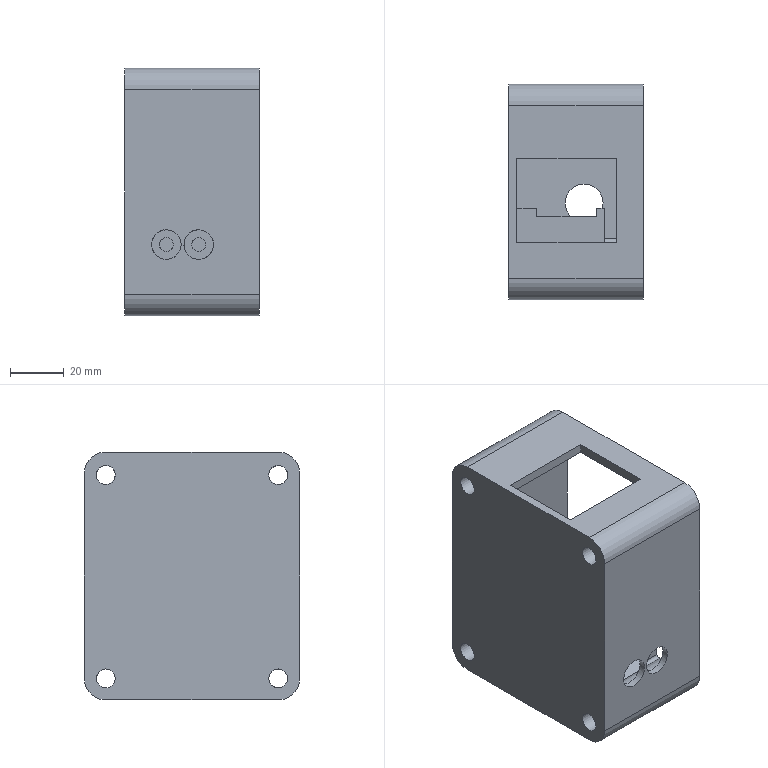NC program | NX | posted by the shop | part box 50 x 80 x 92 mm
Lines 6023 to 6904 of 30419:
(T=7 N=D6-18-D6-50-3T-rough D=6.00 R=0.00 FL=18.00 L=50.00)
(XY-STOCK=0.20)
T7 M6
T11
G0 G90 G54 X34.33 Y-2.568 S4500 M3
G43 H07 Z30.
M8
Z-12.6
G1 X34.203 Y-2.647 Z-13.537 F1500.
X34.075 Y-2.726 Z-13.908
X33.948 Y-2.805 Z-14.18
X33.821 Y-2.884 Z-14.4
X33.693 Y-2.964 Z-14.584
X33.566 Y-3.043 Z-14.742
X33.438 Y-3.122 Z-14.88
X33.311 Y-3.201 Z-15.
X33.184 Y-3.28 Z-15.105
X33.056 Y-3.359 Z-15.198
X32.929 Y-3.439 Z-15.279
X32.801 Y-3.518 Z-15.35
X32.674 Y-3.597 Z-15.41
X32.547 Y-3.676 Z-15.462
X32.419 Y-3.755 Z-15.505
X32.292 Y-3.834 Z-15.539
X32.164 Y-3.914 Z-15.566
X32.037 Y-3.993 Z-15.585
X31.91 Y-4.072 Z-15.596
X31.782 Y-4.151 Z-15.6
X31.004 Y-4.635
G3 X30.803 Y-5.459 I.32 J-.515
X32.656 Y-6.958 I2.88 J1.665
X38.298 Y-4.177 I1.507 J4.056
G1 X38.3 Y-4.147
G3 X38.03 Y-3.647 I-.602 J-.001
G1 X37.795 Y-3.491
X36.799 Y-2.834 Z-15.5
G2 X36.474 Y-2.534 I.395 J.753 F10000.
G1 X36.422 Y-2.396
X36.402 Y-2.25
Y-2.047
X36.411 Y-1.845
G2 X36.787 Y-1.388 I.593 J-.104
X37.582 Y-1.786 Z-15.584 I.214 J-.566 F1500.
G1 X37.649 Y-1.968 Z-15.6
X38.284 Y-3.706
G2 X37.886 Y-5.225 I-2.13 J-.254
X31.206 Y-6.114 I-3.701 J2.265
X30.611 Y-5.298 I1.747 J1.898
X31.515 Y-4.65 I.583 J.141
X31.777 Y-4.97 Z-15.565 I-.44 J-.627
G1 X32.153 Y-5.646 Z-15.5
G3 X33.295 Y-5.298 I.55 J.243 F10000.
X32.764 Y-4.733 I-.618 J-.049
G1 X32.009 Y-4.64
X31.594 Y-4.587 Z-15.535 F1500.
X31.177 Y-4.544 Z-15.57
G3 X30.845 Y-4.655 Z-15.6 I.025 J-.629
X30.598 Y-5.222 I.349 J-.49
X31.213 Y-6.254 I1.851 J.405
X37.298 Y-6.14 I2.983 J3.241
X38.299 Y-4.544 I-2.18 J2.479
G1 X38.3 Y-4.168
G2 X37.808 Y-5.653 I-2.067 J-.138
X31.244 Y-6.371 I-3.609 J2.636
X30.634 Y-5.49 I1.506 J1.696
X31.506 Y-4.849 I.59 J.112
X31.8 Y-5.176 Z-15.563 I-.368 J-.626
G1 X32.174 Y-5.821 Z-15.5
G3 X33.318 Y-5.49 I.546 J.254 F10000.
G1 X33.292 Y-5.303
X33.234 Y-5.122
G3 X32.763 Y-4.797 I-.537 J-.273
G1 X32.036 Y-4.719
X31.184 Y-4.634 Z-15.572 F1500.
G3 X30.868 Y-4.737 Z-15.6 I.031 J-.633
X30.609 Y-5.312 I.338 J-.498
X31.31 Y-6.555 I1.834 J.215
X36.925 Y-6.697 I2.897 J3.466
X38.294 Y-4.934 I-1.965 J2.938
G1 X38.3 Y-4.544
G2 X37.849 Y-5.882 I-1.818 J-.133
X31.367 Y-6.688 I-3.639 J2.797
X30.662 Y-5.711 I1.279 J1.666
G1 X30.64 Y-5.547
G3 X31.372 Y-6.811 I1.799 J.198
X36.481 Y-7.202 I2.846 J3.608
X38.282 Y-5.306 I-1.668 J3.387
G1 X38.3 Y-4.898
G2 X37.866 Y-6.132 I-1.656 J-.111
X31.456 Y-6.961 I-3.641 J2.956
X30.694 Y-5.958 I1.204 J1.704
G1 X30.673 Y-5.795
G3 X31.353 Y-6.991 I1.695 J.171
X35.78 Y-7.717 I2.861 J3.587
X38.222 Y-5.752 I-1.197 J3.986
X38.3 Y-5.201 I-1.014 J.425
G2 X37.856 Y-6.406 I-1.583 J-.101
X31.527 Y-7.213 I-3.614 J3.123
X30.705 Y-6.132 I1.104 J1.693
G1 X30.7 Y-6.088
G2 X31.363 Y-5.473 I.6 J.018
X31.856 Y-5.816 Z-15.548 I-.098 J-.666
G1 X32.184 Y-6.281 Z-15.5
X32.298 Y-6.441 F10000.
X32.437 Y-6.579
G3 X33.384 Y-6.088 I.347 J.489
X32.889 Y-5.412 I-.619 J.065
G1 X32.522 Y-5.4
X32.154 Y-5.402
X31.216 Y-5.407 Z-15.579 F1500.
X31.094 Y-5.44 Z-15.589
X30.979 Y-5.494 Z-15.6
G3 X30.7 Y-6.001 I.323 J-.508
X31.206 Y-7.047 I1.411 J.036
X34.739 Y-8.145 I2.943 J3.238
X38.07 Y-6.292 I-.373 J4.591
X38.3 Y-5.487 I-.883 J.688
G2 X37.848 Y-6.667 I-1.526 J-.092
X31.594 Y-7.457 I-3.59 J3.266
X30.703 Y-6.293 I1.075 J1.745
G1 X30.7 Y-6.132
G3 X31.234 Y-7.269 I1.458 J-.009
X34.709 Y-8.346 I2.926 J3.301
X38.047 Y-6.579 I-.311 J4.625
X38.3 Y-5.762 I-.857 J.713
G2 X37.873 Y-6.881 I-1.447 J-.089
X33.255 Y-8.348 I-3.603 J3.341
X30.926 Y-6.986 I.564 J3.639
X30.7 Y-6.326 I.823 J.65
G3 X31.218 Y-7.446 I1.437 J-.016
X34.57 Y-8.555 I2.938 J3.262
X37.986 Y-6.908 I-.173 J4.724
X38.3 Y-6.029 I-.855 J.802
G2 X37.838 Y-7.161 I-1.447 J-.069
X33.258 Y-8.543 I-3.548 J3.478
X30.929 Y-7.184 I.567 J3.648
X30.7 Y-6.504 I.816 J.654
G3 X31.186 Y-7.607 I1.411 J-.037
X34.351 Y-8.762 I2.95 J3.168
X37.935 Y-7.209 I.042 J4.816
X38.3 Y-6.282 I-.85 J.87
G2 X37.865 Y-7.363 I-1.383 J-.072
X33.974 Y-8.829 I-3.507 J3.413
X31.111 Y-7.608 I.088 J4.174
X30.7 Y-6.708 I.862 J.937
G3 X31.223 Y-7.838 I1.46 J-.01
X34.504 Y-8.957 I2.955 J3.293
X37.925 Y-7.453 I-.066 J4.795
X38.3 Y-6.509 I-.836 J.878
G2 X37.858 Y-7.602 I-1.371 J-.081
X34.098 Y-9.033 I-3.464 J3.447
X31.107 Y-7.797 I-.004 J4.228
X30.7 Y-6.9 I.871 J.936
G3 X31.232 Y-8.04 I1.472 J-.007
X34.505 Y-9.158 I2.964 J3.327
X37.924 Y-7.683 I-.038 J4.789
X38.3 Y-6.757 I-.818 J.871
G2 X37.856 Y-7.831 I-1.351 J-.07
X34.223 Y-9.235 I-3.424 J3.459
X31.173 Y-8.061 I-.077 J4.349
X30.7 Y-7.092 I.885 J1.032
G3 X31.233 Y-8.235 I1.476 J-.007
X34.483 Y-9.36 I2.976 J3.339
X37.903 Y-7.934 I.003 J4.808
X38.3 Y-6.987 I-.812 J.897
G2 X37.851 Y-8.06 I-1.342 J-.069
X34.358 Y-9.437 I-3.382 J3.462
X31.19 Y-8.273 I-.172 J4.424
X30.7 Y-7.403 I1.059 J1.169
G1 Y-7.283
G3 X31.257 Y-8.452 I1.5 J-.003
X34.58 Y-9.558 I2.985 J3.424
X37.906 Y-8.154 I-.056 J4.771
X38.3 Y-7.213 I-.801 J.888
G2 X37.861 Y-8.272 I-1.322 J-.072
X34.424 Y-9.638 I-3.358 J3.444
X31.24 Y-8.517 I-.202 J4.509
X30.7 Y-7.596 I1.057 J1.238
G1 Y-7.476
G3 X31.22 Y-8.61 I1.469 J-.013
X34.435 Y-9.764 I3.01 J3.33
X37.841 Y-8.445 I.076 J4.862
X38.3 Y-7.645 I-.951 J1.077
G1 Y-7.45
G2 X37.853 Y-8.501 I-1.315 J-.061
X34.48 Y-9.839 I-3.323 J3.458
X31.221 Y-8.693 I-.24 J4.525
X30.7 Y-7.792 I1.085 J1.228
G1 Y-7.657
G3 X31.258 Y-8.843 I1.507 J-.015
X34.551 Y-9.964 I3.011 J3.446
X37.882 Y-8.621 I.008 J4.783
X38.3 Y-7.661 I-.788 J.914
G2 X37.852 Y-8.72 I-1.31 J-.07
X34.487 Y-10.041 I-3.301 J3.463
X31.228 Y-8.895 I-.23 J4.552
X30.7 Y-7.989 I1.087 J1.241
G1 Y-7.854
G3 X31.218 Y-8.998 I1.457 J-.029
X34.429 Y-10.169 I3.04 J3.347
X37.836 Y-8.887 I.12 J4.849
X38.3 Y-8.086 I-.927 J1.072
G1 Y-7.891
G2 X37.839 Y-8.95 I-1.311 J-.06
X34.509 Y-10.243 I-3.271 J3.49
X31.249 Y-9.111 I-.23 J4.596
X30.7 Y-8.183 I1.062 J1.255
G1 Y-8.063
G3 X31.222 Y-9.198 I1.475 J-.009
X34.425 Y-10.371 I3.049 J3.364
X37.822 Y-9.117 I.138 J4.855
X38.3 Y-8.311 I-.943 J1.103
G1 Y-8.112
G2 X37.847 Y-9.158 I-1.299 J-.059
X34.528 Y-10.446 I-3.256 J3.472
X31.25 Y-9.307 I-.233 J4.618
X30.7 Y-8.375 I1.082 J1.267
G1 Y-8.255
G3 X31.218 Y-9.389 I1.475 J-.012
X34.427 Y-10.574 I3.066 J3.364
X37.821 Y-9.333 I.152 J4.843
X38.3 Y-8.52 I-.915 J1.086
G1 Y-8.325
G2 X37.843 Y-9.377 I-1.297 J-.062
X34.603 Y-10.648 I-3.227 J3.463
X31.281 Y-9.534 I-.279 J4.677
X30.7 Y-8.575 I1.09 J1.316
G1 Y-8.44
G3 X31.218 Y-9.586 I1.464 J-.028
X34.415 Y-10.777 I3.076 J3.368
X37.832 Y-9.536 I.181 J4.826
X38.3 Y-8.735 I-.902 J1.065
G1 Y-8.54
G2 X37.838 Y-9.596 I-1.297 J-.061
X34.588 Y-10.852 I-3.211 J3.477
X31.257 Y-9.707 I-.259 J4.665
X30.7 Y-8.775 I1.088 J1.282
G1 Y-8.64
G3 X31.208 Y-9.773 I1.46 J-.026
X34.379 Y-10.98 I3.088 J3.344
X37.808 Y-9.773 I.219 J4.848
X38.3 Y-8.949 I-.899 J1.096
G1 Y-8.754
G2 X37.828 Y-9.818 I-1.302 J-.059
X34.513 Y-11.056 I-3.201 J3.514
X31.271 Y-9.918 I-.18 J4.673
X30.7 Y-8.964 I1.07 J1.289
G1 Y-8.829
G3 X31.213 Y-9.975 I1.477 J-.027
X34.423 Y-11.184 I3.103 J3.372
X37.804 Y-9.989 I.192 J4.833
X38.3 Y-9.161 I-.894 J1.098
G1 Y-8.966
G2 X37.829 Y-10.029 I-1.298 J-.061
X34.567 Y-11.259 I-3.183 J3.498
X31.27 Y-10.115 I-.216 J4.698
X30.7 Y-9.158 I1.081 J1.292
G1 Y-9.038
G3 X31.22 Y-10.18 I1.489 J-.011
X34.428 Y-11.388 I3.108 J3.392
X37.826 Y-10.179 I.205 J4.803
X38.3 Y-9.382 I-.906 J1.079
G1 Y-9.187
G2 X37.881 Y-10.186 I-1.239 J-.068
X34.789 Y-11.456 I-3.172 J3.326
X31.302 Y-10.343 I-.396 J4.781
X30.7 Y-9.351 I1.086 J1.338
G1 Y-9.231
G3 X31.253 Y-10.411 I1.522 J-.007
X34.592 Y-11.591 I3.115 J3.501
X37.84 Y-10.375 I.078 J4.738
X38.3 Y-9.589 I-.885 J1.046
G1 Y-9.394
G2 X37.838 Y-10.441 I-1.28 J-.061
X34.664 Y-11.665 I-3.153 J3.452
X31.263 Y-10.504 I-.284 J4.732
X30.7 Y-9.555 I1.113 J1.301
G1 Y-9.42
G3 X31.222 Y-10.578 I1.498 J-.022
X34.455 Y-11.795 I3.128 J3.409
X37.816 Y-10.61 I.2 J4.791
X38.3 Y-9.797 I-.88 J1.075
G1 Y-9.617
G2 X37.877 Y-10.612 I-1.233 J-.063
X34.776 Y-11.865 I-3.153 J3.339
X31.304 Y-10.742 I-.366 J4.798
X30.7 Y-9.753 I1.114 J1.359
G1 Y-9.618
G3 X31.248 Y-10.804 I1.523 J-.015
X34.588 Y-11.999 I3.136 J3.498
X37.843 Y-10.793 I.1 J4.722
X38.3 Y-10.008 I-.874 J1.035
G1 Y-9.813
G2 X37.834 Y-10.865 I-1.281 J-.062
X34.631 Y-12.074 I-3.138 J3.467
X31.268 Y-10.907 I-.237 J4.745
X30.7 Y-9.95 I1.107 J1.305
G1 Y-9.815
G3 X31.224 Y-10.978 I1.505 J-.022
X34.491 Y-12.203 I3.148 J3.427
X37.805 Y-11.039 I.183 J4.777
X38.3 Y-10.222 I-.889 J1.098
G1 Y-10.027
G2 X37.829 Y-11.08 I-1.282 J-.058
X34.634 Y-12.278 I-3.126 J3.478
X31.288 Y-11.125 I-.228 J4.77
X30.7 Y-10.15 I1.107 J1.333
G1 Y-10.015
G3 X31.252 Y-11.206 I1.531 J-.014
X34.594 Y-12.407 I3.148 J3.512
X37.84 Y-11.214 I.11 J4.71
X38.3 Y-10.429 I-.872 J1.039
G1 Y-10.249
G2 X37.836 Y-11.282 I-1.27 J-.05
X34.656 Y-12.482 I-3.12 J3.455
X31.279 Y-11.316 I-.243 J4.774
X30.7 Y-10.346 I1.1 J1.314
G1 Y-10.211
G3 X31.251 Y-11.405 I1.533 J-.017
X34.587 Y-12.611 I3.155 J3.509
X37.84 Y-11.422 I.124 J4.706
X38.3 Y-10.636 I-.863 J1.033
G1 Y-10.456
G2 X37.83 Y-11.496 I-1.276 J-.05
X34.629 Y-12.686 I-3.113 J3.472
X31.27 Y-11.508 I-.214 J4.766
X30.7 Y-10.546 I1.109 J1.307
G1 Y-10.411
G3 X31.247 Y-11.601 I1.531 J-.018
X34.599 Y-12.815 I3.166 J3.507
X37.844 Y-11.626 I.121 J4.692
X38.3 Y-10.848 I-.874 J1.035
G1 Y-10.653
G2 X37.831 Y-11.703 I-1.273 J-.061
X34.641 Y-12.89 I-3.106 J3.466
X31.262 Y-11.7 I-.22 J4.768
X30.7 Y-10.746 I1.117 J1.3
G1 Y-10.611
G3 X31.253 Y-11.808 I1.538 J-.016
X34.611 Y-13.019 I3.168 J3.523
X37.832 Y-11.846 I.113 J4.699
X38.3 Y-11.054 I-.866 J1.047
G1 Y-10.874
G2 X37.832 Y-11.91 I-1.269 J-.05
X34.653 Y-13.094 I-3.099 J3.459
X31.26 Y-11.899 I-.225 J4.774
X30.7 Y-10.953 I1.142 J1.315
G1 Y-10.813
G3 X31.252 Y-12.008 I1.539 J-.014
X34.653 Y-13.223 I3.18 J3.534
X37.832 Y-12.053 I.082 J4.68
X38.3 Y-11.267 I-.873 J1.052
G1 Y-11.072
G2 X37.833 Y-12.116 I-1.268 J-.06
X34.695 Y-13.298 I-3.088 J3.446
X31.294 Y-12.132 I-.25 J4.817
X30.7 Y-11.146 I1.122 J1.347
G1 Y-11.011
G3 X31.246 Y-12.203 I1.536 J-.017
X34.625 Y-13.427 I3.186 J3.518
X37.81 Y-12.282 I.106 J4.706
X38.3 Y-11.48 I-.884 J1.09
G1 Y-11.294
G2 X37.84 Y-12.317 I-1.255 J-.05
X34.717 Y-13.501 I-3.085 J3.425
X31.284 Y-12.324 I-.266 J4.818
X30.7 Y-11.351 I1.126 J1.337
G1 Y-11.216
G3 X31.234 Y-12.392 I1.517 J-.021
X34.566 Y-13.632 I3.192 J3.481
X37.817 Y-12.483 I.162 J4.713
X38.3 Y-11.681 I-.866 J1.069
G1 Y-11.501
G2 X37.876 Y-12.486 I-1.219 J-.059
X34.847 Y-13.701 I-3.084 J3.304
X31.325 Y-12.564 I-.369 J4.882
X30.7 Y-11.554 I1.126 J1.395
G1 Y-11.419
G3 X31.197 Y-12.554 I1.477 J-.03
X34.424 Y-13.834 I3.203 J3.37
X37.796 Y-12.709 I.285 J4.764
X38.3 Y-11.884 I-.861 J1.093
G1 Y-11.704
G2 X37.87 Y-12.698 I-1.227 J-.06
X34.839 Y-13.906 I-3.077 J3.317
X31.3 Y-12.742 I-.362 J4.863
X30.7 Y-11.752 I1.107 J1.347
G1 Y-11.617
G3 X31.218 Y-12.778 I1.511 J-.022
X34.489 Y-14.039 I3.201 J3.43
X37.807 Y-12.905 I.236 J4.733
X38.3 Y-12.092 I-.861 J1.078
G1 Y-11.912
G2 X37.871 Y-12.905 I-1.22 J-.061
X34.86 Y-14.109 I-3.07 J3.308
X31.334 Y-12.977 I-.371 J4.898
X30.7 Y-11.954 I1.121 J1.403
G1 Y-11.819
G3 X31.241 Y-13.004 I1.535 J-.015
X34.628 Y-14.244 I3.206 J3.513
X37.826 Y-13.093 I.124 J4.673
X38.3 Y-12.297 I-.852 J1.046
G1 Y-12.117
G2 X37.877 Y-13.104 I-1.213 J-.065
X34.851 Y-14.314 I-3.072 J3.297
X31.309 Y-13.155 I-.364 J4.879
X30.7 Y-12.153 I1.13 J1.372
G1 Y-12.018
G3 X31.217 Y-13.181 I1.516 J-.023
X34.501 Y-14.448 I3.211 J3.432
X37.818 Y-13.307 I.234 J4.713
X38.3 Y-12.504 I-.854 J1.058
G1 Y-12.324
G2 X37.872 Y-13.316 I-1.217 J-.063
X34.833 Y-14.519 I-3.068 J3.313
X31.306 Y-13.354 I-.345 J4.876
X30.7 Y-12.354 I1.129 J1.367
G1 Y-12.219
G3 X31.249 Y-13.416 I1.546 J-.016
X34.663 Y-14.652 I3.212 J3.537
X37.849 Y-13.483 I.106 J4.634
X38.3 Y-12.716 I-.862 J1.023
G1 Y-12.521
G2 X37.872 Y-13.522 I-1.223 J-.069
X34.824 Y-14.724 I-3.067 J3.315
X31.296 Y-13.546 I-.336 J4.868
X30.7 Y-12.552 I1.132 J1.354
G1 Y-12.417
G3 X31.249 Y-13.619 I1.55 J-.018
X34.631 Y-14.857 I3.21 J3.53
X37.848 Y-13.69 I.136 J4.643
X38.3 Y-12.921 I-.864 J1.026
G1 Y-12.741
G2 X37.878 Y-13.721 I-1.213 J-.059
X34.845 Y-14.927 I-3.066 J3.296
X31.307 Y-13.76 I-.35 J4.884
X30.7 Y-12.757 I1.13 J1.369
G1 Y-12.622
G3 X31.25 Y-13.821 I1.549 J-.016
X34.665 Y-15.061 I3.217 J3.539
X37.82 Y-13.923 I.102 J4.659
X38.3 Y-13.122 I-.852 J1.054
G1 Y-12.942
G2 X37.872 Y-13.933 I-1.215 J-.064
X34.833 Y-15.132 I-3.061 J3.309
X31.297 Y-13.952 I-.339 J4.874
X30.7 Y-12.955 I1.133 J1.355
G1 Y-12.82
G3 X31.25 Y-14.024 I1.552 J-.019
X34.636 Y-15.265 I3.215 J3.533
X37.812 Y-14.136 I.127 J4.674
X38.3 Y-13.334 I-.864 J1.075
G1 Y-13.139
G2 X37.83 Y-14.182 I-1.262 J-.059
X34.688 Y-15.34 I-3.053 J3.443
X31.246 Y-14.104 I-.219 J4.803
X30.7 Y-13.157 I1.134 J1.283
G1 Y-13.022
G3 X31.252 Y-14.229 I1.555 J-.018
X34.657 Y-15.469 I3.218 J3.542
X37.844 Y-14.31 I.121 J4.631
X38.3 Y-13.535 I-.852 J1.023
G1 Y-13.355
G2 X37.873 Y-14.344 I-1.219 J-.06
X34.838 Y-15.54 I-3.056 J3.306
X31.298 Y-14.358 I-.338 J4.879
X30.7 Y-13.362 I1.135 J1.358
G1 Y-13.227
G3 X31.251 Y-14.43 I1.555 J-.017
X34.648 Y-15.673 I3.22 J3.537
X37.828 Y-14.531 I.126 J4.648
X38.3 Y-13.741 I-.853 J1.045
G1 Y-13.561
G2 X37.87 Y-14.552 I-1.22 J-.059
X34.838 Y-15.744 I-3.052 J3.308
X31.308 Y-14.571 I-.335 J4.891
X30.7 Y-13.567 I1.136 J1.374
G1 Y-13.432
G3 X31.245 Y-14.627 I1.548 J-.017
X34.668 Y-15.878 I3.23 J3.532
X37.82 Y-14.745 I.108 J4.65
X38.3 Y-13.945 I-.851 J1.055
G1 Y-13.765
G2 X37.867 Y-14.76 I-1.218 J-.062
X34.819 Y-15.949 I-3.051 J3.321
X31.269 Y-14.737 I-.323 J4.856
X30.7 Y-13.777 I1.161 J1.337
G1 Y-13.637
G3 X31.251 Y-14.837 I1.553 J-.013
X34.68 Y-16.082 I3.228 J3.547
X37.85 Y-14.921 I.108 J4.613
X38.3 Y-14.155 I-.856 J1.019
G1 Y-13.96
G2 X37.873 Y-14.96 I-1.219 J-.07
X34.899 Y-16.15 I-3.04 J3.284
X31.323 Y-14.991 I-.383 J4.915
X30.7 Y-13.972 I1.133 J1.392
G1 Y-13.837
G3 X31.238 Y-15.027 I1.543 J-.019
X34.599 Y-16.286 I3.229 J3.503
X37.829 Y-15.146 I.173 J4.656
X38.3 Y-14.357 I-.852 J1.043
G1 Y-14.177
G2 X37.831 Y-15.208 I-1.26 J-.049
X34.711 Y-16.361 I-3.04 J3.431
X31.267 Y-15.141 I-.225 J4.835
X30.7 Y-14.183 I1.161 J1.334
G1 Y-14.044
G3 X31.251 Y-15.243 I1.555 J-.012
X34.69 Y-16.49 I3.232 J3.551
X37.827 Y-15.353 I.096 J4.632
X38.3 Y-14.561 I-.848 J1.044
G1 Y-14.381
G2 X37.868 Y-15.375 I-1.217 J-.062
X34.831 Y-16.562 I-3.045 J3.315
X31.279 Y-15.356 I-.327 J4.871
X30.7 Y-14.378 I1.132 J1.331
G1 Y-14.243
G3 X31.239 Y-15.434 I1.544 J-.018
X34.621 Y-16.695 I3.235 J3.51
X37.826 Y-15.56 I.158 J4.649
X38.3 Y-14.766 I-.85 J1.046
G1 Y-14.586
G2 X37.873 Y-15.575 I-1.217 J-.061
X34.901 Y-16.763 I-3.036 J3.282
X31.319 Y-15.597 I-.381 J4.917
X30.7 Y-14.586 I1.147 J1.396
G1 Y-14.451
G3 X31.207 Y-15.604 I1.499 J-.029
X34.487 Y-16.897 I3.241 J3.415
X36.669 Y-16.5 I.149 J5.368
X37.828 Y-15.757 I-2.293 J4.853
X38.3 Y-14.975 I-.848 J1.045
G1 Y-14.795
G2 X37.833 Y-15.814 I-1.237 J-.05
X36.832 Y-16.404 I-1.55 J1.489
G3 X37.997 Y-15.749 I-.637 J2.496
X38.3 Y-14.994 I-.643 J.697
G2 X37.785 Y-15.999 I-1.143 J-.049
X37.375 Y-16.202 I-.897 J1.301
G3 X38.291 Y-15.393 I-.245 J1.201
G1 X38.3 Y-15.175
G2 X37.681 Y-16.088 I-.882 J-.068
G3 X38.3 Y-15.318 I-.143 J.749
G2 X37.938 Y-15.98 I-.683 J-.056
G3 X38.252 Y-15.631 I-.265 J.554
G2 X37.898 Y-16.001 I-.598 J.218
G3 X36.318 Y-16.676 I2.778 J-8.686
G2 X31.385 Y-15.861 I-1.747 J4.763
X30.7 Y-14.793 I1.137 J1.482
G1 Y-14.658
G3 X31.207 Y-15.807 I1.495 J-.027
X34.526 Y-17.1 I3.243 J3.416
X36. Y-16.895 I.121 J4.529
G1 X36.572 Y-16.557
G2 X34.278 Y-17.163 I-1.934 J2.677
X31.16 Y-15.843 I.106 J4.592
X30.7 Y-14.992 I1.127 J1.158
G1 Y-14.857
G3 X31.245 Y-16.051 I1.547 J-.016
X35.657 Y-17.132 I3.178 J3.428
G1 X35.772 Y-17.061
G3 X35.973 Y-16.522 I-.395 J.454
G1 X35.654 Y-15.372 Z-15.5
X35.588 Y-15.147 F10000.
X35.535 Y-14.919
G2 X35.772 Y-14.377 I.598 J.061
G1 X36.052 Y-14.178
G2 X36.794 Y-14.339 I.272 J-.535
X36.862 Y-14.985 Z-15.557 I-.485 J-.378 F1500.
G1 X36.676 Y-15.457 Z-15.6
X36.218 Y-16.619
G2 X35.965 Y-16.916 I-.567 J.227
X34.709 Y-17.352 I-1.203 J1.437
X31.167 Y-16.054 I-.331 J4.58
X30.7 Y-15.2 I1.167 J1.192
G1 Y-15.06
G3 X31.251 Y-16.261 I1.555 J-.013
X35.391 Y-17.34 I3.047 J3.211
X35.753 Y-17.077 I-.969 J1.713
G2 X34.56 Y-17.533 I-1.134 J1.181
X31.089 Y-16.168 I-.29 J4.359
X30.7 Y-15.266 I.918 J.93
G3 X31.231 Y-16.443 I1.525 J-.02
X35.14 Y-17.538 I2.951 J3.011
X35.543 Y-17.258 I-.562 J1.238
G2 X34.344 Y-17.709 I-1.112 J1.139
X31. Y-16.26 I-.198 J4.124
X30.7 Y-15.471 I.889 J.79
G3 X31.199 Y-16.612 I1.491 J-.028
X34.879 Y-17.733 I2.873 J2.833
X35.325 Y-17.445 I-.35 J1.033
G2 X34.133 Y-17.877 I-1.076 J1.11
X30.975 Y-16.428 I-.099 J3.95
X30.7 Y-15.668 I.875 J.746
G3 X31.255 Y-16.872 I1.551 J-.015
X34.679 Y-17.904 I2.691 J2.731
X35.013 Y-17.725 I-.271 J.907
X35.164 Y-17.094 I-.46 J.443
X34.756 Y-16.674 Z-15.549 I-.628 J-.202
G1 X34.219 Y-16.44 Z-15.5
X32.198 Y-15.558 F10000.
X31.848 Y-15.402 Z-15.532 F1500.
X31.492 Y-15.26 Z-15.564
G3 X31.076 Y-15.297 Z-15.6 I-.152 J-.644
X30.7 Y-15.878 I.263 J-.582
X31.344 Y-17.077 I1.695 J.139
X34.556 Y-18.025 I2.559 J2.757
X34.948 Y-17.809 I-.206 J.84
X35.062 Y-17.19 I-.515 J.416
X34.605 Y-16.746 Z-15.545 I-.692 J-.255
G1 X34.122 Y-16.522 Z-15.5
X32.197 Y-15.629 F10000.
X31.875 Y-15.478 Z-15.53 F1500.
X31.548 Y-15.336 Z-15.56
G3 X31.08 Y-15.371 Z-15.6 I-.186 J-.653
X30.7 Y-15.968 I.281 J-.598
X31.308 Y-17.161 I1.662 J.096
X34.498 Y-18.124 I2.524 J2.591
X35.051 Y-17.682 I-.267 J.902
G1 X35.119 Y-17.623
G2 X34.721 Y-18.045 I-9.598 J8.648
X33.031 Y-18.151 I-.986 J2.192
X30.826 Y-16.616 I.65 J3.285
X30.7 Y-16.087 I.869 J.485
G3 X31.276 Y-17.329 I1.589 J-.018
X34.307 Y-18.286 I2.446 J2.467
X34.855 Y-17.924 I-.145 J.815
G2 X33.949 Y-18.383 I-.897 J.645
X30.838 Y-16.844 I-.279 J3.35
X30.7 Y-16.286 I.85 J.506
G3 X31.245 Y-17.496 I1.541 J-.033
X34.243 Y-18.416 I2.344 J2.292
X34.738 Y-18.068 I-.188 J.792
G2 X33.776 Y-18.534 I-.924 J.684
X30.84 Y-17.05 I-.207 J3.237
X30.7 Y-16.507 I.836 J.505
G3 X31.256 Y-17.701 I1.526 J-.016
X34.125 Y-18.56 I2.229 J2.221
X34.619 Y-18.214 I-.188 J.795
G2 X33.655 Y-18.678 I-.925 J.689
X30.797 Y-17.165 I-.203 J3.072
X30.7 Y-16.715 I.87 J.422
G3 X31.249 Y-17.884 I1.498 J-.01
X34.066 Y-18.685 I2.121 J2.103
X34.506 Y-18.354 I-.244 J.781
G2 X33.689 Y-18.8 I-.858 J.6
X30.86 Y-17.476 I-.298 J3.049
X30.7 Y-16.898 I.828 J.539
G3 X31.259 Y-18.08 I1.482 J-.023
X32.617 Y-18.8 I1.938 J2.013
G1 X33.187
G2 X31.96 Y-18.623 I-.271 J2.453
X30.707 Y-17.294 I.828 J2.035
G1 X30.7 Y-17.1
G3 X31.011 Y-17.986 I1.224 J-.068
X32.227 Y-18.797 I1.911 J1.545
G1 X32.575 Y-18.8
G2 X31.309 Y-18.284 I-.175 J1.381
G3 X31.963 Y-18.778 I1.215 J.926
G1 X32.238 Y-18.8
G2 X31.61 Y-18.584 I-.073 J.809
X30.796 Y-17.701 I3.355 J3.91
X30.7 Y-17.295 I.842 J.412
G3 X30.96 Y-17.934 I.792 J-.051
G1 X31.61 Y-18.584
G3 X32.133 Y-18.8 I.528 J.538
X33.938 Y-18.781 I.561 J33.079
X34.352 Y-18.537 I-.191 J.797
X34.43 Y-17.802 I-.44 J.418
G1 X33.828 Y-16.822
X33.749 Y-16.694 Z-15.596
X33.67 Y-16.566 Z-15.585
X33.592 Y-16.439 Z-15.566
X33.513 Y-16.311 Z-15.539
X33.435 Y-16.183 Z-15.505
X33.356 Y-16.055 Z-15.462
X33.278 Y-15.928 Z-15.41
X33.199 Y-15.8 Z-15.35
X33.121 Y-15.672 Z-15.279
X33.042 Y-15.544 Z-15.198
X32.964 Y-15.416 Z-15.105
X32.885 Y-15.289 Z-15.
X32.806 Y-15.161 Z-14.88
X32.728 Y-15.033 Z-14.742
X32.649 Y-14.905 Z-14.584
X32.571 Y-14.777 Z-14.4
X32.492 Y-14.65 Z-14.18
X32.414 Y-14.522 Z-13.908
X32.335 Y-14.394 Z-13.537
X32.257 Y-14.266 Z-12.6
G0 Z30.
X34.745 Y-12.455
Z-10.65
G1 X34.802 Y-12.593 Z-11.587
X34.859 Y-12.732 Z-11.958
X34.917 Y-12.871 Z-12.23
X34.974 Y-13.009 Z-12.45
X35.032 Y-13.148 Z-12.634
X35.089 Y-13.286 Z-12.792
X35.146 Y-13.425 Z-12.93
X35.204 Y-13.563 Z-13.05
X35.261 Y-13.702 Z-13.155
X35.319 Y-13.841 Z-13.248
X35.376 Y-13.979 Z-13.329
X35.434 Y-14.118 Z-13.4
X35.491 Y-14.256 Z-13.46
X35.548 Y-14.395 Z-13.512
X35.606 Y-14.533 Z-13.555
X35.663 Y-14.672 Z-13.589
X35.721 Y-14.811 Z-13.616
X35.778 Y-14.949 Z-13.635
X35.836 Y-15.088 Z-13.646
X35.893 Y-15.226 Z-13.65
X36.182 Y-15.923
G3 X37.12 Y-16.164 I.56 J.232
X38.3 Y-14.419 I-1.803 J2.49
X37.692 Y-13.742 I-.66 J.019
X37.072 Y-14.059 Z-13.589 I-.047 J-.674
G1 X36.802 Y-14.432 Z-13.55
X36.42 Y-14.959 F10000.
X36.14 Y-15.357 Z-13.591 F1500.
G3 X36.18 Y-16.028 Z-13.65 I.595 J-.301
X37.11 Y-16.197 I.547 J.37
X38.298 Y-14.694 I-1.191 J2.163
G1 X38.3 Y-14.124
G2 X38.224 Y-15.007 I-2.222 J-.253
X37.142 Y-16.285 I-2.735 J1.216
X36.258 Y-15.887 I-.274 J.571
X36.436 Y-15.238 Z-13.591 I.669 J.166
G1 X36.737 Y-14.854 Z-13.55
X36.788 Y-14.788 F10000.
X37.006 Y-14.507 Z-13.58 F1500.
X37.232 Y-14.233 Z-13.61
G2 X37.669 Y-14.061 Z-13.65 I.441 J-.479
X38.3 Y-14.694 I-.003 J-.634
X37.592 Y-15.997 I-2.016 J.252
G1 X37.295 Y-16.23
G2 X36.5 Y-15.27 I-.268 J.587
G1 X37.128 Y-14.382
G2 X38.3 Y-14.754 I.527 J-.372
X37.408 Y-16.189 I-1.917 J.197
X36.606 Y-15.226 I-.243 J.614
G1 X37.08 Y-14.465
G2 X38.3 Y-14.814 I.56 J-.349
X37.529 Y-16.143 I-1.737 J.12
X36.699 Y-15.217 I-.267 J.596
G1 X36.916 Y-14.841
X37.145 Y-14.473
G2 X38.3 Y-14.889 I.502 J-.417
X37.638 Y-16.1 I-1.568 J.071
X36.809 Y-15.227 I-.279 J.565
G1 X36.988 Y-14.903
X37.178 Y-14.586
G2 X38.3 Y-14.979 I.492 J-.394
X37.717 Y-16.07 I-1.37 J.031
X36.876 Y-15.217 I-.282 J.563
G1 X37.014 Y-14.942
X37.167 Y-14.675
G2 X38.3 Y-15.054 I.503 J-.379
X37.787 Y-16.044 I-1.198 J-.006
X36.938 Y-15.214 I-.285 J.558
G1 X37.045 Y-14.988
X37.163 Y-14.767
G2 X38.3 Y-15.129 I.511 J-.362
X37.842 Y-16.023 I-1.049 J-.026
X36.984 Y-15.206 I-.288 J.556
G1 X37.156 Y-14.852
G2 X38.3 Y-15.204 I.518 J-.352
X37.9 Y-15.998 I-.918 J-.035
X36.989 Y-15.195 I-.305 J.573
X37.225 Y-14.79 I.872 J-.237
X38.3 Y-15.279 I.426 J-.489
X37.961 Y-15.967 I-.8 J-.033
X36.98 Y-15.337 I-.321 J.579
X38.3 Y-15.339 I.66 J-.003
X37.825 Y-16.034 I-.686 J-.041
G1 X36.939 Y-16.364
X37.898 Y-16.001
G3 X38.256 Y-15.617 I-.241 J.584
X37.765 Y-14.834 I-.578 J.183
G1 X36.794 Y-14.694
X36.646 Y-14.672 Z-13.646
X36.497 Y-14.651 Z-13.635
X36.349 Y-14.629 Z-13.616
X36.2 Y-14.608 Z-13.589
X36.052 Y-14.587 Z-13.555
X35.903 Y-14.565 Z-13.512
X35.755 Y-14.544 Z-13.46
X35.606 Y-14.522 Z-13.4
X35.458 Y-14.501 Z-13.329
X35.31 Y-14.48 Z-13.248
X35.161 Y-14.458 Z-13.155
X35.013 Y-14.437 Z-13.05
X34.864 Y-14.415 Z-12.93
X34.716 Y-14.394 Z-12.792
X34.567 Y-14.372 Z-12.634
X34.419 Y-14.351 Z-12.45
X34.27 Y-14.33 Z-12.23
X34.122 Y-14.308 Z-11.958
X33.973 Y-14.287 Z-11.587
X33.825 Y-14.265 Z-10.65
G0 Z30.
X35.422 Y-17.843
Z-4.3
G1 X35.445 Y-17.991 Z-5.237
X35.469 Y-18.139 Z-5.608
X35.492 Y-18.288 Z-5.88
X35.515 Y-18.436 Z-6.1
X35.538 Y-18.584 Z-6.284
X35.561 Y-18.732 Z-6.442
X35.584 Y-18.88 Z-6.58
X35.607 Y-19.029 Z-6.7
X35.631 Y-19.177 Z-6.805
X35.654 Y-19.325 Z-6.898
X35.677 Y-19.473 Z-6.979
X35.7 Y-19.622 Z-7.05
X35.723 Y-19.77 Z-7.11
X35.746 Y-19.918 Z-7.162
X35.77 Y-20.066 Z-7.205
X35.793 Y-20.214 Z-7.239
X35.816 Y-20.363 Z-7.266
X35.839 Y-20.511 Z-7.285
X35.862 Y-20.659 Z-7.296
X35.885 Y-20.807 Z-7.3
X36.039 Y-21.788
G3 X36.636 Y-22.3 I.599 J.094
X39.101 Y-20.814 I-.516 J3.644
X39.8 Y-19.43 I-2.555 J2.16
X39.329 Y-18.799 I-.661 J-.001
X38.66 Y-18.975 Z-7.239 I-.187 J-.649
G1 X38.31 Y-19.283 Z-7.2
X36.59 Y-20.8 F10000.
X36.132 Y-21.214 Z-7.252 F1500.
G3 X35.985 Y-21.752 Z-7.3 I.515 J-.429
X36.636 Y-22.3 I.651 J.112
X38.57 Y-21.528 I-.019 J2.857
X39.795 Y-19.782 I-2.372 J2.967
G1 X39.8 Y-19.122
G2 X39.728 Y-20.067 I-2.586 J-.277
X37.193 Y-22.299 I-3.432 J1.341
G1 X36.863 Y-22.3
G3 X38.712 Y-21.632 I.15 J2.475
X39.795 Y-20.105 I-1.934 J2.521
G1 X39.8 Y-19.754
G2 X39.342 Y-21.064 I-1.783 J-.112
X37.531 Y-22.3 I-2.547 J1.786
G1 X37.276
G3 X38.906 Y-21.678 I.101 J2.183
X39.798 Y-20.385 I-1.52 J2.002
G1 X39.8 Y-20.07
G2 X39.313 Y-21.349 I-1.653 J-.104
X37.829 Y-22.3 I-2.079 J1.611
G1 X37.619
G3 X39.153 Y-21.658 I.068 J1.99
X39.8 Y-20.631 I-1.203 J1.474
G1 Y-20.378
G2 X39.342 Y-21.536 I-1.463 J-.091
X38.099 Y-22.3 I-1.716 J1.397
G1 X37.919
G3 X39.36 Y-21.645 I.052 J1.799
X39.8 Y-20.856 I-.962 J1.055
G1 Y-20.646
G2 X39.297 Y-21.772 I-1.359 J-.068
X38.345 Y-22.3 I-1.317 J1.251
G1 X38.18
G3 X39.585 Y-21.561 I.04 J1.628
X39.8 Y-20.885 I-.693 J.593
G2 X39.315 Y-21.912 I-1.205 J-.059
X38.407 Y-22.3 I-.906 J.865
G3 X39.799 Y-21.266 I.07 J1.36
G1 X39.8 Y-21.093
G2 X39.267 Y-22.077 I-1.094 J-.044
X38.62 Y-22.3 I-.626 J.766
G3 X39.8 Y-21.397 I.081 J1.117
G1 Y-21.262
G2 X39.203 Y-22.209 I-.986 J-.039
X38.791 Y-22.3 I-.391 J.787
G3 X39.8 Y-21.523 I.086 J.932
G1 Y-21.403
G2 X38.951 Y-22.3 I-.846 J-.05
G3 X39.8 Y-21.53 I.083 J.762